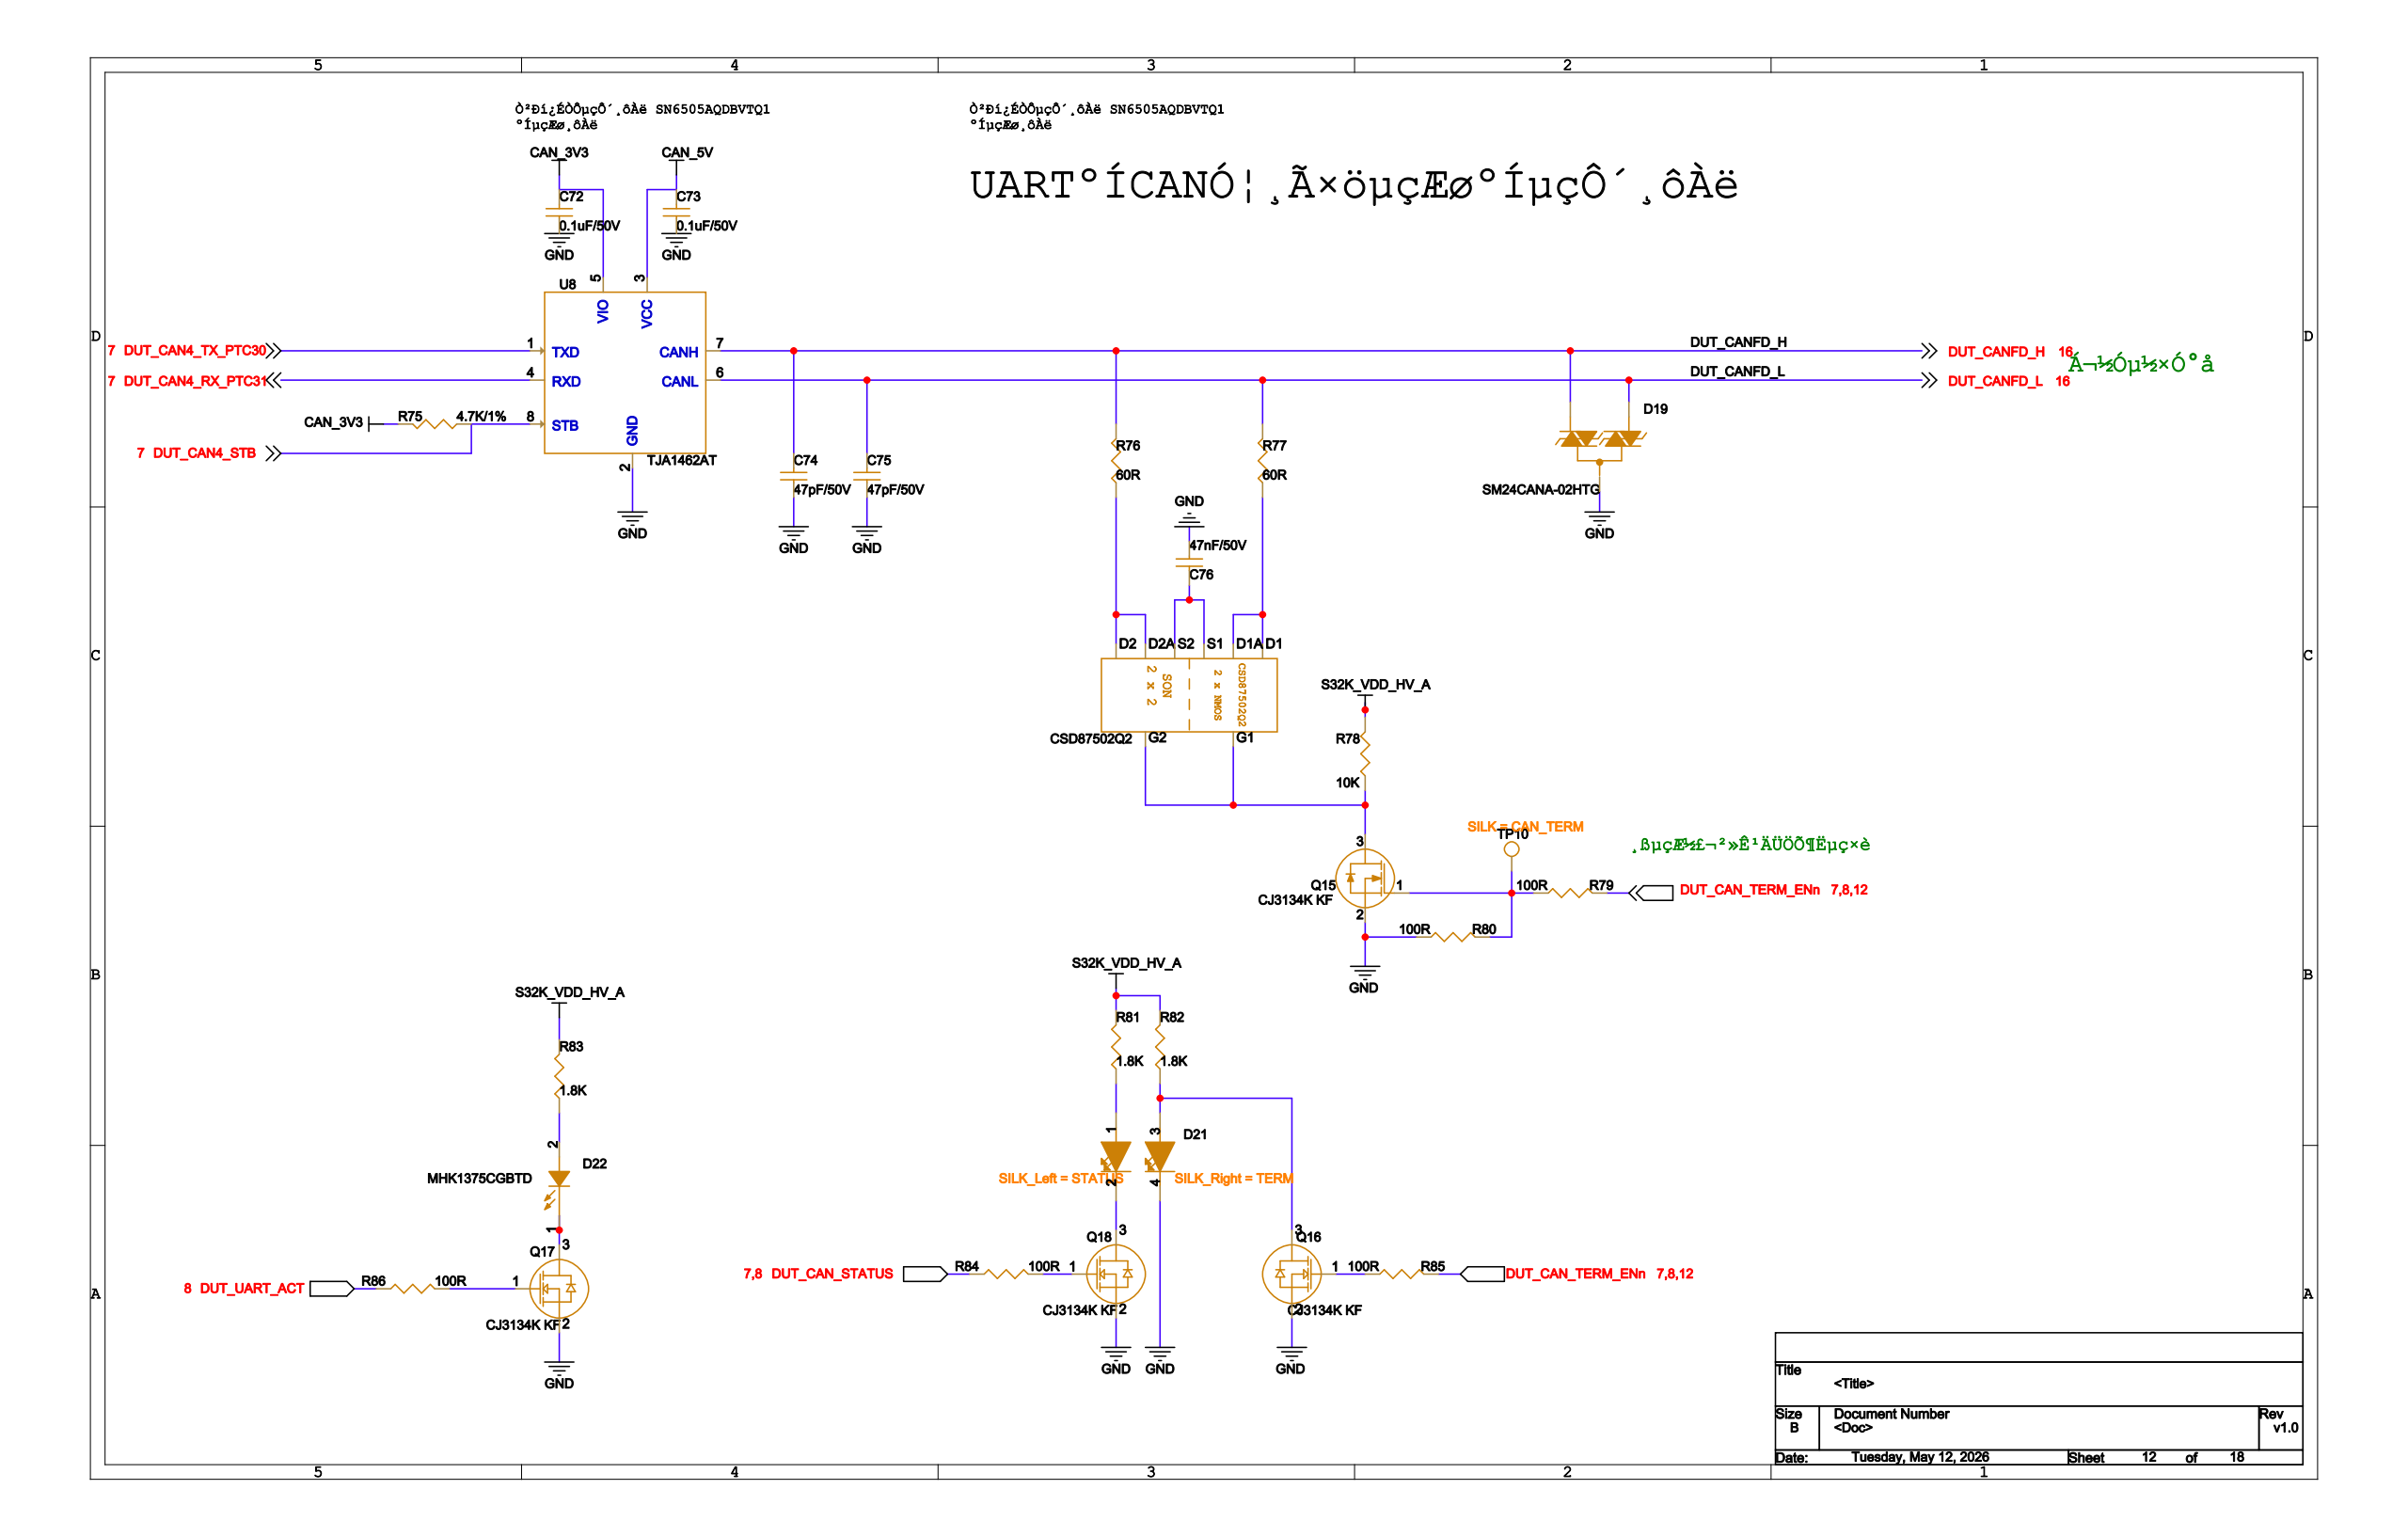Circuit board | Cadence Allegro | 330 parts | 215 nets | one sheet of the schematic
Parts on this sheet (reference | value | footprint):
C72 | 0.1uF/50V | C0402
C73 | 0.1uF/50V | C0402
C74 | 47pF/50V | C0402
C75 | 47pF/50V | C0402
C76 | 47nF/50V | C0402
D19 | SM24CANA-02HTG | SOT23-3
D21 | MHK2396YGBTD | LED_D3_WX2
D22 | MHK1375CGBTD | LED-TH_MHK1375CRBTD
Q15 | CJ3134K KF | SOT723
Q16 | CJ3134K KF | SOT-723
Q17 | CJ3134K KF | SOT-723
Q18 | CJ3134K KF | SOT-723
R75 | 4.7K/1% | R0402
R76 | 60R | R0402
R77 | 60R | R0402
R78 | 10K | 0402
R79 | 100R | 0402
R80 | 100R | 0402
R81 | 1.8K | 0402
R82 | 1.8K | 0402
R83 | 1.8K | 0402
R84 | 100R | 0402
R85 | 100R | 0402
R86 | 100R | 0402
TP10 | TP | S0400CI
U8 | TJA1462AT | SO8
Nets of these parts (net: part-pin ...):
GND: C72-1 C73-1 C74-1 C75-1 C76-1 D19-3 D21-4 Q15-2 Q16-2 Q17-2 Q18-2 R80-2 U8-2
DUT_CANFD_H: C74-2 D19-2 R76-1 U8-7
DUT_CANFD_L: C75-2 D19-1 R77-1 U8-6
CAN_3V3: C72-2 R75-1 U8-5
DUT_CAN4_STB: R75-2 U8-8
N16958314: R76-2
N16958316: R77-2
S32K_VDD_HV_A: R78-2 R81-2 R82-2 R83-2
CAN_5V: C73-2 U8-3
N16958343: C76-2
N16944920: D22-1 Q17-3
N16944906: D22-2 R83-1
N16921257: D21-1 R81-1
N16959685: D21-2 Q18-3
N16960203: D21-3 Q16-3 R82-1
N16960121: Q16-1 R85-2
N16944946: Q17-1 R86-2
N16921335: Q18-1 R84-2
N16958390: Q15-3 R78-1
DUT_CAN4_RX_PTC31: U8-4
DUT_CAN4_TX_PTC30: U8-1
DUT_CAN_STATUS: R84-1
DUT_CAN_TERM_ENN: R79-1 R85-1
DUT_UART_ACT: R86-1
N16958425: Q15-1 R79-2 R80-1 TP10-1